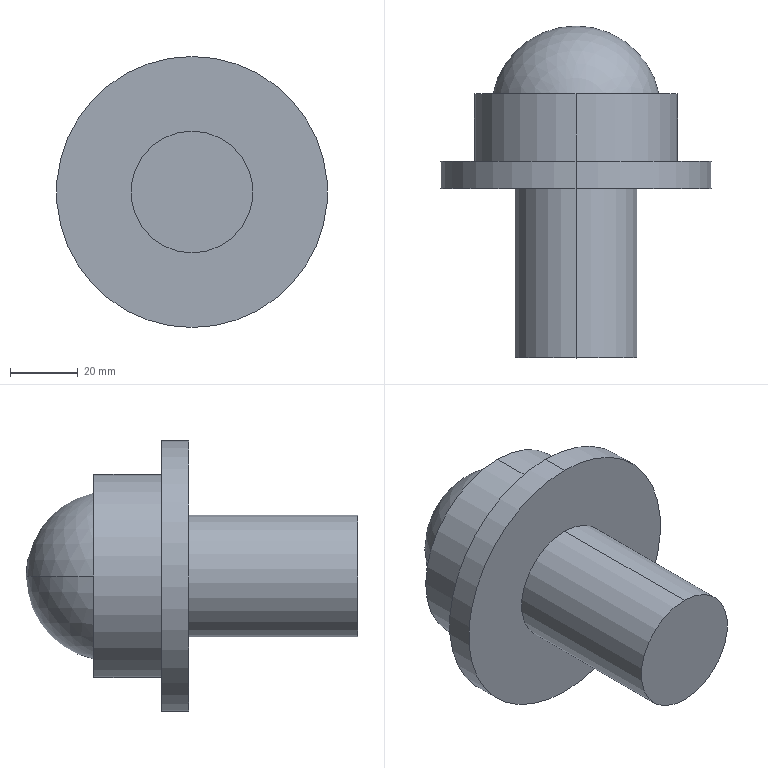Part | SolidWorks | features ICE 1, Revolution 1 | 1 solid | 12 faces | box 80 x 98 x 80 mm | volume 170693 mm3 | cylinder 6 | plane 4 | sphere 2 | commonest cylinder face diameters 36 x2 60 x2 80 x2
STEP:
#1=CARTESIAN_POINT('',(0.,-50.,-18.));
#2=VERTEX_POINT('',#1);
#3=CARTESIAN_POINT('',(0.,-50.,18.));
#4=VERTEX_POINT('',#3);
#5=CARTESIAN_POINT('',(0.,-50.,0.));
#6=DIRECTION('',(0.,-1.,0.));
#7=DIRECTION('',(0.,0.,-1.));
#8=AXIS2_PLACEMENT_3D('',#5,#6,#7);
#9=CIRCLE('',#8,18.);
#10=EDGE_CURVE('',#2,#4,#9,.T.);
#11=ORIENTED_EDGE('',*,*,#10,.F.);
#12=CARTESIAN_POINT('',(0.,0.,-18.));
#13=VERTEX_POINT('',#12);
#14=CARTESIAN_POINT('',(0.,-50.,-18.));
#15=DIRECTION('',(0.,1.,0.));
#16=VECTOR('',#15,1000.);
#17=LINE('',#14,#16);
#18=EDGE_CURVE('',#2,#13,#17,.T.);
#19=ORIENTED_EDGE('',*,*,#18,.T.);
#20=CARTESIAN_POINT('',(0.,0.,18.));
#21=VERTEX_POINT('',#20);
#22=CARTESIAN_POINT('',(0.,0.,0.));
#23=DIRECTION('',(0.,-1.,0.));
#24=DIRECTION('',(0.,0.,-1.));
#25=AXIS2_PLACEMENT_3D('',#22,#23,#24);
#26=CIRCLE('',#25,18.);
#27=EDGE_CURVE('',#13,#21,#26,.T.);
#28=ORIENTED_EDGE('',*,*,#27,.T.);
#29=CARTESIAN_POINT('',(0.,-50.,18.));
#30=DIRECTION('',(0.,1.,0.));
#31=VECTOR('',#30,1000.);
#32=LINE('',#29,#31);
#33=EDGE_CURVE('',#4,#21,#32,.T.);
#34=ORIENTED_EDGE('',*,*,#33,.F.);
#35=EDGE_LOOP('',(#11,#19,#28,#34));
#36=FACE_OUTER_BOUND('',#35,.T.);
#37=CARTESIAN_POINT('',(0.,-50.,0.));
#38=DIRECTION('',(0.,1.,0.));
#39=DIRECTION('',(0.,0.,1.));
#40=AXIS2_PLACEMENT_3D('',#37,#38,#39);
#41=CYLINDRICAL_SURFACE('',#40,18.);
#42=ADVANCED_FACE('',(#36),#41,.T.);
#43=CARTESIAN_POINT('',(0.,8.,-40.));
#44=VERTEX_POINT('',#43);
#45=CARTESIAN_POINT('',(0.,8.,40.));
#46=VERTEX_POINT('',#45);
#47=CARTESIAN_POINT('',(0.,8.,0.));
#48=DIRECTION('',(0.,-1.,0.));
#49=DIRECTION('',(0.,0.,-1.));
#50=AXIS2_PLACEMENT_3D('',#47,#48,#49);
#51=CIRCLE('',#50,40.);
#52=EDGE_CURVE('',#44,#46,#51,.T.);
#53=ORIENTED_EDGE('',*,*,#52,.T.);
#54=CARTESIAN_POINT('',(0.,0.,40.));
#55=VERTEX_POINT('',#54);
#56=CARTESIAN_POINT('',(0.,0.,40.));
#57=DIRECTION('',(0.,-1.,0.));
#58=VECTOR('',#57,1000.);
#59=LINE('',#56,#58);
#60=EDGE_CURVE('',#46,#55,#59,.T.);
#61=ORIENTED_EDGE('',*,*,#60,.T.);
#62=CARTESIAN_POINT('',(0.,0.,-40.));
#63=VERTEX_POINT('',#62);
#64=CARTESIAN_POINT('',(0.,0.,0.));
#65=DIRECTION('',(0.,-1.,0.));
#66=DIRECTION('',(0.,0.,-1.));
#67=AXIS2_PLACEMENT_3D('',#64,#65,#66);
#68=CIRCLE('',#67,40.);
#69=EDGE_CURVE('',#63,#55,#68,.T.);
#70=ORIENTED_EDGE('',*,*,#69,.F.);
#71=CARTESIAN_POINT('',(0.,0.,-40.));
#72=DIRECTION('',(0.,-1.,0.));
#73=VECTOR('',#72,1000.);
#74=LINE('',#71,#73);
#75=EDGE_CURVE('',#44,#63,#74,.T.);
#76=ORIENTED_EDGE('',*,*,#75,.F.);
#77=EDGE_LOOP('',(#53,#61,#70,#76));
#78=FACE_OUTER_BOUND('',#77,.T.);
#79=CARTESIAN_POINT('',(0.,0.,0.));
#80=DIRECTION('',(0.,-1.,0.));
#81=DIRECTION('',(0.,0.,-1.));
#82=AXIS2_PLACEMENT_3D('',#79,#80,#81);
#83=CYLINDRICAL_SURFACE('',#82,40.);
#84=ADVANCED_FACE('',(#78),#83,.T.);
#85=CARTESIAN_POINT('',(0.,28.,-30.));
#86=VERTEX_POINT('',#85);
#87=CARTESIAN_POINT('',(0.,28.,30.));
#88=VERTEX_POINT('',#87);
#89=CARTESIAN_POINT('',(0.,28.,0.));
#90=DIRECTION('',(0.,-1.,0.));
#91=DIRECTION('',(0.,0.,-1.));
#92=AXIS2_PLACEMENT_3D('',#89,#90,#91);
#93=CIRCLE('',#92,30.);
#94=EDGE_CURVE('',#86,#88,#93,.T.);
#95=ORIENTED_EDGE('',*,*,#94,.T.);
#96=CARTESIAN_POINT('',(0.,8.,30.));
#97=VERTEX_POINT('',#96);
#98=CARTESIAN_POINT('',(0.,0.,30.));
#99=DIRECTION('',(0.,-1.,0.));
#100=VECTOR('',#99,1000.);
#101=LINE('',#98,#100);
#102=EDGE_CURVE('',#88,#97,#101,.T.);
#103=ORIENTED_EDGE('',*,*,#102,.T.);
#104=CARTESIAN_POINT('',(0.,8.,-30.));
#105=VERTEX_POINT('',#104);
#106=CARTESIAN_POINT('',(0.,8.,0.));
#107=DIRECTION('',(0.,-1.,0.));
#108=DIRECTION('',(0.,0.,-1.));
#109=AXIS2_PLACEMENT_3D('',#106,#107,#108);
#110=CIRCLE('',#109,30.);
#111=EDGE_CURVE('',#105,#97,#110,.T.);
#112=ORIENTED_EDGE('',*,*,#111,.F.);
#113=CARTESIAN_POINT('',(0.,0.,-30.));
#114=DIRECTION('',(0.,-1.,0.));
#115=VECTOR('',#114,1000.);
#116=LINE('',#113,#115);
#117=EDGE_CURVE('',#86,#105,#116,.T.);
#118=ORIENTED_EDGE('',*,*,#117,.F.);
#119=EDGE_LOOP('',(#95,#103,#112,#118));
#120=FACE_OUTER_BOUND('',#119,.T.);
#121=CARTESIAN_POINT('',(0.,0.,0.));
#122=DIRECTION('',(0.,-1.,0.));
#123=DIRECTION('',(0.,0.,-1.));
#124=AXIS2_PLACEMENT_3D('',#121,#122,#123);
#125=CYLINDRICAL_SURFACE('',#124,30.);
#126=ADVANCED_FACE('',(#120),#125,.T.);
#127=CARTESIAN_POINT('',(0.,48.,0.));
#128=VERTEX_POINT('',#127);
#129=CARTESIAN_POINT('',(24.495,28.,0.));
#130=VERTEX_POINT('',#129);
#131=CARTESIAN_POINT('',(0.,23.,0.));
#132=DIRECTION('',(0.,0.,-1.));
#133=DIRECTION('',(-1.,0.,0.));
#134=AXIS2_PLACEMENT_3D('',#131,#132,#133);
#135=CIRCLE('',#134,25.);
#136=EDGE_CURVE('',#128,#130,#135,.T.);
#137=ORIENTED_EDGE('',*,*,#136,.F.);
#138=CARTESIAN_POINT('',(-24.495,28.,0.));
#139=VERTEX_POINT('',#138);
#140=CARTESIAN_POINT('',(0.,23.,0.));
#141=DIRECTION('',(0.,0.,1.));
#142=DIRECTION('',(1.,0.,0.));
#143=AXIS2_PLACEMENT_3D('',#140,#141,#142);
#144=CIRCLE('',#143,25.);
#145=EDGE_CURVE('',#128,#139,#144,.T.);
#146=ORIENTED_EDGE('',*,*,#145,.T.);
#147=CARTESIAN_POINT('',(0.,28.,0.));
#148=DIRECTION('',(0.,-1.,0.));
#149=DIRECTION('',(0.,0.,-1.));
#150=AXIS2_PLACEMENT_3D('',#147,#148,#149);
#151=CIRCLE('',#150,24.495);
#152=EDGE_CURVE('',#130,#139,#151,.T.);
#153=ORIENTED_EDGE('',*,*,#152,.F.);
#154=EDGE_LOOP('',(#137,#146,#153));
#155=FACE_OUTER_BOUND('',#154,.T.);
#156=CARTESIAN_POINT('',(0.,23.,0.));
#157=DIRECTION('',(0.,0.,1.));
#158=DIRECTION('',(1.,0.,0.));
#159=AXIS2_PLACEMENT_3D('',#156,#157,#158);
#160=SPHERICAL_SURFACE('',#159,25.);
#161=ADVANCED_FACE('',(#155),#160,.T.);
#162=ORIENTED_EDGE('',*,*,#145,.F.);
#163=ORIENTED_EDGE('',*,*,#136,.T.);
#164=CARTESIAN_POINT('',(0.,28.,0.));
#165=DIRECTION('',(0.,-1.,0.));
#166=DIRECTION('',(0.,0.,-1.));
#167=AXIS2_PLACEMENT_3D('',#164,#165,#166);
#168=CIRCLE('',#167,24.495);
#169=EDGE_CURVE('',#139,#130,#168,.T.);
#170=ORIENTED_EDGE('',*,*,#169,.F.);
#171=EDGE_LOOP('',(#162,#163,#170));
#172=FACE_OUTER_BOUND('',#171,.T.);
#173=CARTESIAN_POINT('',(0.,23.,0.));
#174=DIRECTION('',(0.,0.,1.));
#175=DIRECTION('',(1.,0.,0.));
#176=AXIS2_PLACEMENT_3D('',#173,#174,#175);
#177=SPHERICAL_SURFACE('',#176,25.);
#178=ADVANCED_FACE('',(#172),#177,.T.);
#179=ORIENTED_EDGE('',*,*,#94,.F.);
#180=CARTESIAN_POINT('',(0.,28.,0.));
#181=DIRECTION('',(0.,-1.,0.));
#182=DIRECTION('',(0.,0.,-1.));
#183=AXIS2_PLACEMENT_3D('',#180,#181,#182);
#184=CIRCLE('',#183,30.);
#185=EDGE_CURVE('',#88,#86,#184,.T.);
#186=ORIENTED_EDGE('',*,*,#185,.F.);
#187=EDGE_LOOP('',(#179,#186));
#188=FACE_OUTER_BOUND('',#187,.T.);
#189=ORIENTED_EDGE('',*,*,#152,.T.);
#190=ORIENTED_EDGE('',*,*,#169,.T.);
#191=EDGE_LOOP('',(#189,#190));
#192=FACE_BOUND('',#191,.T.);
#193=CARTESIAN_POINT('',(-24.495,28.,0.));
#194=DIRECTION('',(0.,-1.,0.));
#195=DIRECTION('',(0.,0.,-1.));
#196=AXIS2_PLACEMENT_3D('',#193,#194,#195);
#197=PLANE('',#196);
#198=ADVANCED_FACE('',(#188,#192),#197,.F.);
#199=ORIENTED_EDGE('',*,*,#102,.F.);
#200=ORIENTED_EDGE('',*,*,#185,.T.);
#201=ORIENTED_EDGE('',*,*,#117,.T.);
#202=CARTESIAN_POINT('',(0.,8.,0.));
#203=DIRECTION('',(0.,-1.,0.));
#204=DIRECTION('',(0.,0.,-1.));
#205=AXIS2_PLACEMENT_3D('',#202,#203,#204);
#206=CIRCLE('',#205,30.);
#207=EDGE_CURVE('',#97,#105,#206,.T.);
#208=ORIENTED_EDGE('',*,*,#207,.F.);
#209=EDGE_LOOP('',(#199,#200,#201,#208));
#210=FACE_OUTER_BOUND('',#209,.T.);
#211=CARTESIAN_POINT('',(0.,0.,0.));
#212=DIRECTION('',(0.,-1.,0.));
#213=DIRECTION('',(0.,0.,-1.));
#214=AXIS2_PLACEMENT_3D('',#211,#212,#213);
#215=CYLINDRICAL_SURFACE('',#214,30.);
#216=ADVANCED_FACE('',(#210),#215,.T.);
#217=ORIENTED_EDGE('',*,*,#52,.F.);
#218=CARTESIAN_POINT('',(0.,8.,0.));
#219=DIRECTION('',(0.,-1.,0.));
#220=DIRECTION('',(0.,0.,-1.));
#221=AXIS2_PLACEMENT_3D('',#218,#219,#220);
#222=CIRCLE('',#221,40.);
#223=EDGE_CURVE('',#46,#44,#222,.T.);
#224=ORIENTED_EDGE('',*,*,#223,.F.);
#225=EDGE_LOOP('',(#217,#224));
#226=FACE_OUTER_BOUND('',#225,.T.);
#227=ORIENTED_EDGE('',*,*,#111,.T.);
#228=ORIENTED_EDGE('',*,*,#207,.T.);
#229=EDGE_LOOP('',(#227,#228));
#230=FACE_BOUND('',#229,.T.);
#231=CARTESIAN_POINT('',(-30.,8.,0.));
#232=DIRECTION('',(0.,-1.,0.));
#233=DIRECTION('',(0.,0.,-1.));
#234=AXIS2_PLACEMENT_3D('',#231,#232,#233);
#235=PLANE('',#234);
#236=ADVANCED_FACE('',(#226,#230),#235,.F.);
#237=ORIENTED_EDGE('',*,*,#60,.F.);
#238=ORIENTED_EDGE('',*,*,#223,.T.);
#239=ORIENTED_EDGE('',*,*,#75,.T.);
#240=CARTESIAN_POINT('',(0.,0.,0.));
#241=DIRECTION('',(0.,-1.,0.));
#242=DIRECTION('',(0.,0.,-1.));
#243=AXIS2_PLACEMENT_3D('',#240,#241,#242);
#244=CIRCLE('',#243,40.);
#245=EDGE_CURVE('',#55,#63,#244,.T.);
#246=ORIENTED_EDGE('',*,*,#245,.F.);
#247=EDGE_LOOP('',(#237,#238,#239,#246));
#248=FACE_OUTER_BOUND('',#247,.T.);
#249=CARTESIAN_POINT('',(0.,0.,0.));
#250=DIRECTION('',(0.,-1.,0.));
#251=DIRECTION('',(0.,0.,-1.));
#252=AXIS2_PLACEMENT_3D('',#249,#250,#251);
#253=CYLINDRICAL_SURFACE('',#252,40.);
#254=ADVANCED_FACE('',(#248),#253,.T.);
#255=CARTESIAN_POINT('',(0.,0.,0.));
#256=DIRECTION('',(0.,-1.,0.));
#257=DIRECTION('',(0.,0.,-1.));
#258=AXIS2_PLACEMENT_3D('',#255,#256,#257);
#259=CIRCLE('',#258,18.);
#260=EDGE_CURVE('',#21,#13,#259,.T.);
#261=ORIENTED_EDGE('',*,*,#260,.F.);
#262=ORIENTED_EDGE('',*,*,#27,.F.);
#263=EDGE_LOOP('',(#261,#262));
#264=FACE_BOUND('',#263,.T.);
#265=ORIENTED_EDGE('',*,*,#69,.T.);
#266=ORIENTED_EDGE('',*,*,#245,.T.);
#267=EDGE_LOOP('',(#265,#266));
#268=FACE_OUTER_BOUND('',#267,.T.);
#269=CARTESIAN_POINT('',(-40.,0.,0.));
#270=DIRECTION('',(0.,1.,0.));
#271=DIRECTION('',(0.,0.,1.));
#272=AXIS2_PLACEMENT_3D('',#269,#270,#271);
#273=PLANE('',#272);
#274=ADVANCED_FACE('',(#264,#268),#273,.F.);
#275=ORIENTED_EDGE('',*,*,#18,.F.);
#276=CARTESIAN_POINT('',(0.,-50.,0.));
#277=DIRECTION('',(0.,-1.,0.));
#278=DIRECTION('',(0.,0.,-1.));
#279=AXIS2_PLACEMENT_3D('',#276,#277,#278);
#280=CIRCLE('',#279,18.);
#281=EDGE_CURVE('',#4,#2,#280,.T.);
#282=ORIENTED_EDGE('',*,*,#281,.F.);
#283=ORIENTED_EDGE('',*,*,#33,.T.);
#284=ORIENTED_EDGE('',*,*,#260,.T.);
#285=EDGE_LOOP('',(#275,#282,#283,#284));
#286=FACE_OUTER_BOUND('',#285,.T.);
#287=CARTESIAN_POINT('',(0.,-50.,0.));
#288=DIRECTION('',(0.,1.,0.));
#289=DIRECTION('',(0.,0.,1.));
#290=AXIS2_PLACEMENT_3D('',#287,#288,#289);
#291=CYLINDRICAL_SURFACE('',#290,18.);
#292=ADVANCED_FACE('',(#286),#291,.T.);
#293=ORIENTED_EDGE('',*,*,#281,.T.);
#294=ORIENTED_EDGE('',*,*,#10,.T.);
#295=EDGE_LOOP('',(#293,#294));
#296=FACE_OUTER_BOUND('',#295,.T.);
#297=CARTESIAN_POINT('',(0.,-50.,0.));
#298=DIRECTION('',(0.,-1.,0.));
#299=DIRECTION('',(0.,0.,-1.));
#300=AXIS2_PLACEMENT_3D('',#297,#298,#299);
#301=PLANE('',#300);
#302=ADVANCED_FACE('',(#296),#301,.T.);
#303=CLOSED_SHELL('',(#42,#84,#126,#161,#178,#198,#216,#236,#254,#274,#292,#302));
#304=MANIFOLD_SOLID_BREP('',#303);
#305=CARTESIAN_POINT('',(0.,0.,0.));
#306=DIRECTION('',(0.,0.,1.));
#307=DIRECTION('',(1.,0.,0.));
#308=AXIS2_PLACEMENT_3D('',#305,#306,#307);
#309=(LENGTH_UNIT()NAMED_UNIT(*)SI_UNIT(.MILLI.,.METRE.));
#310=UNCERTAINTY_MEASURE_WITH_UNIT(LENGTH_MEASURE(0.00001),#309,'','');
#311=(NAMED_UNIT(*)PLANE_ANGLE_UNIT()SI_UNIT($,.RADIAN.));
#312=(NAMED_UNIT(*)SI_UNIT($,.STERADIAN.)SOLID_ANGLE_UNIT());
#313=(GEOMETRIC_REPRESENTATION_CONTEXT(3)GLOBAL_UNCERTAINTY_ASSIGNED_CONTEXT((#310))GLOBAL_UNIT_ASSIGNED_CONTEXT((#309,#311,#312))REPRESENTATION_CONTEXT('',''));
#314=ADVANCED_BREP_SHAPE_REPRESENTATION('',(#304,#308),#313);